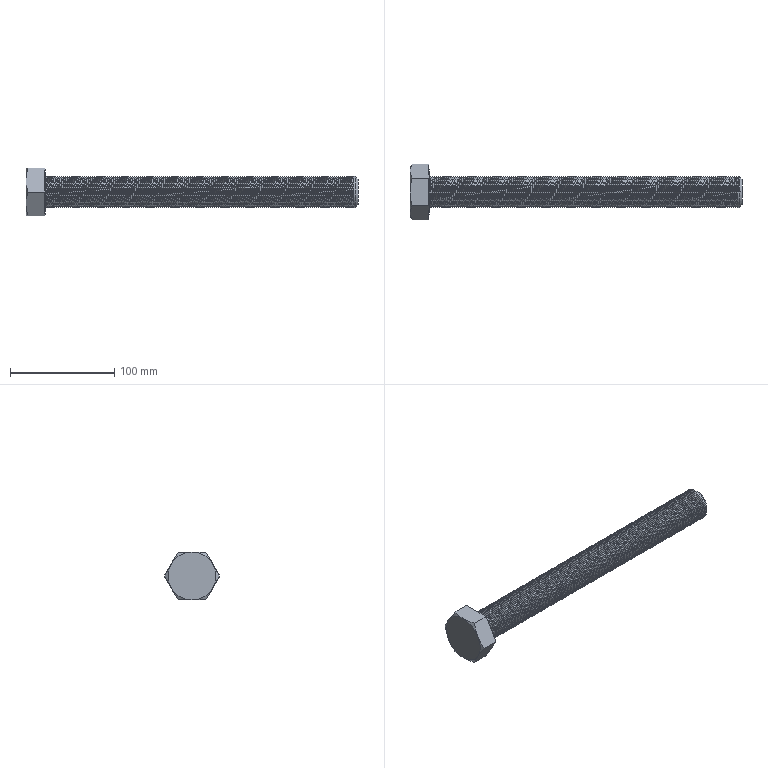Part | SolidWorks | features RevCut 3, Chamfer 1, Extrusion 1, Fillet 1, LPattern 1, Revolution 1, SweepThread 1 | 1 solid | 330 faces | box 318.7 x 53.116 x 46 mm | volume 228448 mm3 | cylinder 303 | plane 12 | cone 10 | spline 3 | torus 2 | commonest cylinder face diameters 30 x303